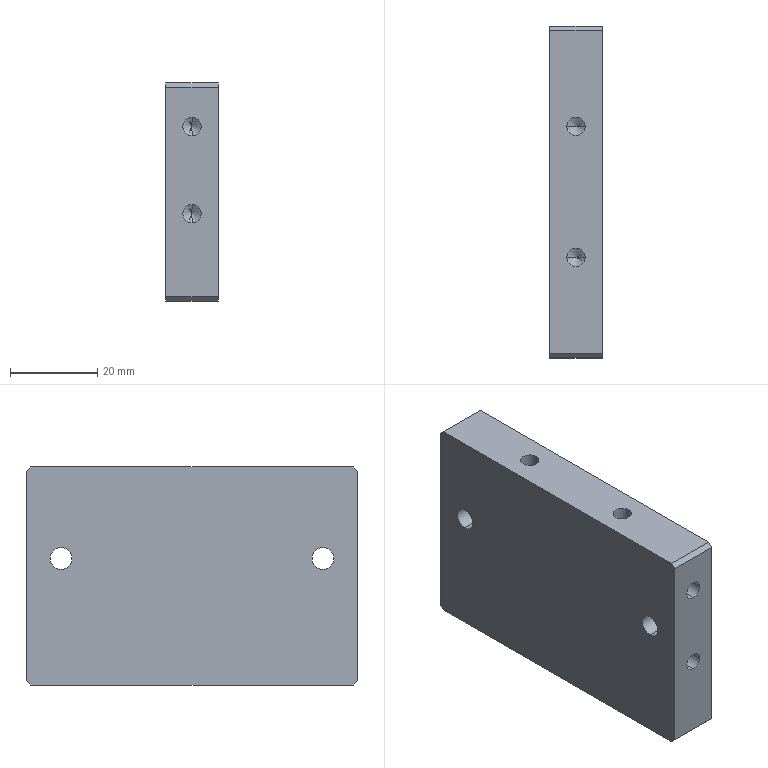Part | SolidWorks | features HoleWzd 3, Chamfer 1, ICE 1, MirrorPattern 1 | 1 solid | 38 faces | box 12 x 76 x 50 mm | volume 43762 mm3 | cylinder 16 | cone 12 | plane 10 | commonest cylinder face diameters 4.2 x12 5 x4
STEP:
#1=CARTESIAN_POINT('',(-8.1,15.,-12.4));
#2=VERTEX_POINT('',#1);
#3=CARTESIAN_POINT('',(-3.9,15.,-12.4));
#4=VERTEX_POINT('',#3);
#5=CARTESIAN_POINT('',(-6.,15.,-12.4));
#6=DIRECTION('',(0.,0.,1.));
#7=DIRECTION('',(1.,0.,0.));
#8=AXIS2_PLACEMENT_3D('',#5,#6,#7);
#9=CIRCLE('',#8,2.1);
#10=EDGE_CURVE('',#2,#4,#9,.T.);
#11=ORIENTED_EDGE('',*,*,#10,.F.);
#12=CARTESIAN_POINT('',(-8.1,15.,0.));
#13=VERTEX_POINT('',#12);
#14=CARTESIAN_POINT('',(-8.1,15.,0.));
#15=DIRECTION('',(0.,0.,1.));
#16=VECTOR('',#15,1000.);
#17=LINE('',#14,#16);
#18=EDGE_CURVE('',#2,#13,#17,.T.);
#19=ORIENTED_EDGE('',*,*,#18,.T.);
#20=CARTESIAN_POINT('',(-3.9,15.,0.));
#21=VERTEX_POINT('',#20);
#22=CARTESIAN_POINT('',(-6.,15.,0.));
#23=DIRECTION('',(0.,0.,1.));
#24=DIRECTION('',(1.,0.,0.));
#25=AXIS2_PLACEMENT_3D('',#22,#23,#24);
#26=CIRCLE('',#25,2.1);
#27=EDGE_CURVE('',#13,#21,#26,.T.);
#28=ORIENTED_EDGE('',*,*,#27,.T.);
#29=CARTESIAN_POINT('',(-3.9,15.,0.));
#30=DIRECTION('',(0.,0.,1.));
#31=VECTOR('',#30,1000.);
#32=LINE('',#29,#31);
#33=EDGE_CURVE('',#4,#21,#32,.T.);
#34=ORIENTED_EDGE('',*,*,#33,.F.);
#35=EDGE_LOOP('',(#11,#19,#28,#34));
#36=FACE_OUTER_BOUND('',#35,.T.);
#37=CARTESIAN_POINT('',(-6.,15.,0.));
#38=DIRECTION('',(0.,0.,1.));
#39=DIRECTION('',(1.,0.,0.));
#40=AXIS2_PLACEMENT_3D('',#37,#38,#39);
#41=CYLINDRICAL_SURFACE('',#40,2.1);
#42=ADVANCED_FACE('',(#36),#41,.F.);
#43=CARTESIAN_POINT('',(-6.,15.,-13.662));
#44=VERTEX_POINT('',#43);
#45=CARTESIAN_POINT('',(-3.9,15.,-12.4));
#46=DIRECTION('',(0.8572,0.,0.515));
#47=VECTOR('',#46,1000.);
#48=LINE('',#45,#47);
#49=EDGE_CURVE('',#44,#4,#48,.T.);
#50=ORIENTED_EDGE('',*,*,#49,.F.);
#51=CARTESIAN_POINT('',(-8.1,15.,-12.4));
#52=DIRECTION('',(-0.8572,0.,0.515));
#53=VECTOR('',#52,1000.);
#54=LINE('',#51,#53);
#55=EDGE_CURVE('',#44,#2,#54,.T.);
#56=ORIENTED_EDGE('',*,*,#55,.T.);
#57=ORIENTED_EDGE('',*,*,#10,.T.);
#58=EDGE_LOOP('',(#50,#56,#57));
#59=FACE_OUTER_BOUND('',#58,.T.);
#60=CARTESIAN_POINT('',(-6.,15.,-12.4));
#61=DIRECTION('',(0.,0.,1.));
#62=DIRECTION('',(1.,0.,0.));
#63=AXIS2_PLACEMENT_3D('',#60,#61,#62);
#64=CONICAL_SURFACE('',#63,2.1,1.03);
#65=ADVANCED_FACE('',(#59),#64,.F.);
#66=CARTESIAN_POINT('',(-8.1,-15.,-12.4));
#67=VERTEX_POINT('',#66);
#68=CARTESIAN_POINT('',(-3.9,-15.,-12.4));
#69=VERTEX_POINT('',#68);
#70=CARTESIAN_POINT('',(-6.,-15.,-12.4));
#71=DIRECTION('',(0.,0.,1.));
#72=DIRECTION('',(1.,0.,0.));
#73=AXIS2_PLACEMENT_3D('',#70,#71,#72);
#74=CIRCLE('',#73,2.1);
#75=EDGE_CURVE('',#67,#69,#74,.T.);
#76=ORIENTED_EDGE('',*,*,#75,.F.);
#77=CARTESIAN_POINT('',(-8.1,-15.,0.));
#78=VERTEX_POINT('',#77);
#79=CARTESIAN_POINT('',(-8.1,-15.,0.));
#80=DIRECTION('',(0.,0.,1.));
#81=VECTOR('',#80,1000.);
#82=LINE('',#79,#81);
#83=EDGE_CURVE('',#67,#78,#82,.T.);
#84=ORIENTED_EDGE('',*,*,#83,.T.);
#85=CARTESIAN_POINT('',(-3.9,-15.,0.));
#86=VERTEX_POINT('',#85);
#87=CARTESIAN_POINT('',(-6.,-15.,0.));
#88=DIRECTION('',(0.,0.,1.));
#89=DIRECTION('',(1.,0.,0.));
#90=AXIS2_PLACEMENT_3D('',#87,#88,#89);
#91=CIRCLE('',#90,2.1);
#92=EDGE_CURVE('',#78,#86,#91,.T.);
#93=ORIENTED_EDGE('',*,*,#92,.T.);
#94=CARTESIAN_POINT('',(-3.9,-15.,0.));
#95=DIRECTION('',(0.,0.,1.));
#96=VECTOR('',#95,1000.);
#97=LINE('',#94,#96);
#98=EDGE_CURVE('',#69,#86,#97,.T.);
#99=ORIENTED_EDGE('',*,*,#98,.F.);
#100=EDGE_LOOP('',(#76,#84,#93,#99));
#101=FACE_OUTER_BOUND('',#100,.T.);
#102=CARTESIAN_POINT('',(-6.,-15.,0.));
#103=DIRECTION('',(0.,0.,1.));
#104=DIRECTION('',(1.,0.,0.));
#105=AXIS2_PLACEMENT_3D('',#102,#103,#104);
#106=CYLINDRICAL_SURFACE('',#105,2.1);
#107=ADVANCED_FACE('',(#101),#106,.F.);
#108=CARTESIAN_POINT('',(-6.,-15.,-13.662));
#109=VERTEX_POINT('',#108);
#110=CARTESIAN_POINT('',(-3.9,-15.,-12.4));
#111=DIRECTION('',(0.8572,0.,0.515));
#112=VECTOR('',#111,1000.);
#113=LINE('',#110,#112);
#114=EDGE_CURVE('',#109,#69,#113,.T.);
#115=ORIENTED_EDGE('',*,*,#114,.F.);
#116=CARTESIAN_POINT('',(-8.1,-15.,-12.4));
#117=DIRECTION('',(-0.8572,0.,0.515));
#118=VECTOR('',#117,1000.);
#119=LINE('',#116,#118);
#120=EDGE_CURVE('',#109,#67,#119,.T.);
#121=ORIENTED_EDGE('',*,*,#120,.T.);
#122=ORIENTED_EDGE('',*,*,#75,.T.);
#123=EDGE_LOOP('',(#115,#121,#122));
#124=FACE_OUTER_BOUND('',#123,.T.);
#125=CARTESIAN_POINT('',(-6.,-15.,-12.4));
#126=DIRECTION('',(0.,0.,1.));
#127=DIRECTION('',(1.,0.,0.));
#128=AXIS2_PLACEMENT_3D('',#125,#126,#127);
#129=CONICAL_SURFACE('',#128,2.1,1.03);
#130=ADVANCED_FACE('',(#124),#129,.F.);
#131=CARTESIAN_POINT('',(-6.,20.6,-12.1));
#132=VERTEX_POINT('',#131);
#133=CARTESIAN_POINT('',(-6.,20.6,-7.9));
#134=VERTEX_POINT('',#133);
#135=CARTESIAN_POINT('',(-6.,20.6,-10.));
#136=DIRECTION('',(0.,1.,0.));
#137=DIRECTION('',(0.,0.,1.));
#138=AXIS2_PLACEMENT_3D('',#135,#136,#137);
#139=CIRCLE('',#138,2.1);
#140=EDGE_CURVE('',#132,#134,#139,.T.);
#141=ORIENTED_EDGE('',*,*,#140,.F.);
#142=CARTESIAN_POINT('',(-6.,38.,-12.1));
#143=VERTEX_POINT('',#142);
#144=CARTESIAN_POINT('',(-6.,38.,-12.1));
#145=DIRECTION('',(0.,1.,0.));
#146=VECTOR('',#145,1000.);
#147=LINE('',#144,#146);
#148=EDGE_CURVE('',#132,#143,#147,.T.);
#149=ORIENTED_EDGE('',*,*,#148,.T.);
#150=CARTESIAN_POINT('',(-6.,38.,-7.9));
#151=VERTEX_POINT('',#150);
#152=CARTESIAN_POINT('',(-6.,38.,-10.));
#153=DIRECTION('',(0.,1.,0.));
#154=DIRECTION('',(0.,0.,1.));
#155=AXIS2_PLACEMENT_3D('',#152,#153,#154);
#156=CIRCLE('',#155,2.1);
#157=EDGE_CURVE('',#143,#151,#156,.T.);
#158=ORIENTED_EDGE('',*,*,#157,.T.);
#159=CARTESIAN_POINT('',(-6.,38.,-7.9));
#160=DIRECTION('',(0.,1.,0.));
#161=VECTOR('',#160,1000.);
#162=LINE('',#159,#161);
#163=EDGE_CURVE('',#134,#151,#162,.T.);
#164=ORIENTED_EDGE('',*,*,#163,.F.);
#165=EDGE_LOOP('',(#141,#149,#158,#164));
#166=FACE_OUTER_BOUND('',#165,.T.);
#167=CARTESIAN_POINT('',(-6.,38.,-10.));
#168=DIRECTION('',(0.,1.,0.));
#169=DIRECTION('',(0.,0.,1.));
#170=AXIS2_PLACEMENT_3D('',#167,#168,#169);
#171=CYLINDRICAL_SURFACE('',#170,2.1);
#172=ADVANCED_FACE('',(#166),#171,.F.);
#173=CARTESIAN_POINT('',(-6.,19.338,-10.));
#174=VERTEX_POINT('',#173);
#175=CARTESIAN_POINT('',(-6.,20.6,-7.9));
#176=DIRECTION('',(0.,0.515,0.8572));
#177=VECTOR('',#176,1000.);
#178=LINE('',#175,#177);
#179=EDGE_CURVE('',#174,#134,#178,.T.);
#180=ORIENTED_EDGE('',*,*,#179,.F.);
#181=CARTESIAN_POINT('',(-6.,20.6,-12.1));
#182=DIRECTION('',(0.,0.515,-0.8572));
#183=VECTOR('',#182,1000.);
#184=LINE('',#181,#183);
#185=EDGE_CURVE('',#174,#132,#184,.T.);
#186=ORIENTED_EDGE('',*,*,#185,.T.);
#187=ORIENTED_EDGE('',*,*,#140,.T.);
#188=EDGE_LOOP('',(#180,#186,#187));
#189=FACE_OUTER_BOUND('',#188,.T.);
#190=CARTESIAN_POINT('',(-6.,20.6,-10.));
#191=DIRECTION('',(0.,1.,0.));
#192=DIRECTION('',(0.,0.,1.));
#193=AXIS2_PLACEMENT_3D('',#190,#191,#192);
#194=CONICAL_SURFACE('',#193,2.1,1.03);
#195=ADVANCED_FACE('',(#189),#194,.F.);
#196=CARTESIAN_POINT('',(-6.,20.6,-32.1));
#197=VERTEX_POINT('',#196);
#198=CARTESIAN_POINT('',(-6.,20.6,-27.9));
#199=VERTEX_POINT('',#198);
#200=CARTESIAN_POINT('',(-6.,20.6,-30.));
#201=DIRECTION('',(0.,1.,0.));
#202=DIRECTION('',(0.,0.,1.));
#203=AXIS2_PLACEMENT_3D('',#200,#201,#202);
#204=CIRCLE('',#203,2.1);
#205=EDGE_CURVE('',#197,#199,#204,.T.);
#206=ORIENTED_EDGE('',*,*,#205,.F.);
#207=CARTESIAN_POINT('',(-6.,38.,-32.1));
#208=VERTEX_POINT('',#207);
#209=CARTESIAN_POINT('',(-6.,38.,-32.1));
#210=DIRECTION('',(0.,1.,0.));
#211=VECTOR('',#210,1000.);
#212=LINE('',#209,#211);
#213=EDGE_CURVE('',#197,#208,#212,.T.);
#214=ORIENTED_EDGE('',*,*,#213,.T.);
#215=CARTESIAN_POINT('',(-6.,38.,-27.9));
#216=VERTEX_POINT('',#215);
#217=CARTESIAN_POINT('',(-6.,38.,-30.));
#218=DIRECTION('',(0.,1.,0.));
#219=DIRECTION('',(0.,0.,1.));
#220=AXIS2_PLACEMENT_3D('',#217,#218,#219);
#221=CIRCLE('',#220,2.1);
#222=EDGE_CURVE('',#208,#216,#221,.T.);
#223=ORIENTED_EDGE('',*,*,#222,.T.);
#224=CARTESIAN_POINT('',(-6.,38.,-27.9));
#225=DIRECTION('',(0.,1.,0.));
#226=VECTOR('',#225,1000.);
#227=LINE('',#224,#226);
#228=EDGE_CURVE('',#199,#216,#227,.T.);
#229=ORIENTED_EDGE('',*,*,#228,.F.);
#230=EDGE_LOOP('',(#206,#214,#223,#229));
#231=FACE_OUTER_BOUND('',#230,.T.);
#232=CARTESIAN_POINT('',(-6.,38.,-30.));
#233=DIRECTION('',(0.,1.,0.));
#234=DIRECTION('',(0.,0.,1.));
#235=AXIS2_PLACEMENT_3D('',#232,#233,#234);
#236=CYLINDRICAL_SURFACE('',#235,2.1);
#237=ADVANCED_FACE('',(#231),#236,.F.);
#238=CARTESIAN_POINT('',(-6.,19.338,-30.));
#239=VERTEX_POINT('',#238);
#240=CARTESIAN_POINT('',(-6.,20.6,-27.9));
#241=DIRECTION('',(0.,0.515,0.8572));
#242=VECTOR('',#241,1000.);
#243=LINE('',#240,#242);
#244=EDGE_CURVE('',#239,#199,#243,.T.);
#245=ORIENTED_EDGE('',*,*,#244,.F.);
#246=CARTESIAN_POINT('',(-6.,20.6,-32.1));
#247=DIRECTION('',(0.,0.515,-0.8572));
#248=VECTOR('',#247,1000.);
#249=LINE('',#246,#248);
#250=EDGE_CURVE('',#239,#197,#249,.T.);
#251=ORIENTED_EDGE('',*,*,#250,.T.);
#252=ORIENTED_EDGE('',*,*,#205,.T.);
#253=EDGE_LOOP('',(#245,#251,#252));
#254=FACE_OUTER_BOUND('',#253,.T.);
#255=CARTESIAN_POINT('',(-6.,20.6,-30.));
#256=DIRECTION('',(0.,1.,0.));
#257=DIRECTION('',(0.,0.,1.));
#258=AXIS2_PLACEMENT_3D('',#255,#256,#257);
#259=CONICAL_SURFACE('',#258,2.1,1.03);
#260=ADVANCED_FACE('',(#254),#259,.F.);
#261=CARTESIAN_POINT('',(-6.,-20.6,-7.9));
#262=VERTEX_POINT('',#261);
#263=CARTESIAN_POINT('',(-6.,-20.6,-12.1));
#264=VERTEX_POINT('',#263);
#265=CARTESIAN_POINT('',(-6.,-20.6,-10.));
#266=DIRECTION('',(0.,-1.,0.));
#267=DIRECTION('',(0.,0.,-1.));
#268=AXIS2_PLACEMENT_3D('',#265,#266,#267);
#269=CIRCLE('',#268,2.1);
#270=EDGE_CURVE('',#262,#264,#269,.T.);
#271=ORIENTED_EDGE('',*,*,#270,.F.);
#272=CARTESIAN_POINT('',(-6.,-38.,-7.9));
#273=VERTEX_POINT('',#272);
#274=CARTESIAN_POINT('',(-6.,-38.,-7.9));
#275=DIRECTION('',(0.,-1.,0.));
#276=VECTOR('',#275,1000.);
#277=LINE('',#274,#276);
#278=EDGE_CURVE('',#262,#273,#277,.T.);
#279=ORIENTED_EDGE('',*,*,#278,.T.);
#280=CARTESIAN_POINT('',(-6.,-38.,-12.1));
#281=VERTEX_POINT('',#280);
#282=CARTESIAN_POINT('',(-6.,-38.,-10.));
#283=DIRECTION('',(0.,-1.,0.));
#284=DIRECTION('',(0.,0.,-1.));
#285=AXIS2_PLACEMENT_3D('',#282,#283,#284);
#286=CIRCLE('',#285,2.1);
#287=EDGE_CURVE('',#273,#281,#286,.T.);
#288=ORIENTED_EDGE('',*,*,#287,.T.);
#289=CARTESIAN_POINT('',(-6.,-38.,-12.1));
#290=DIRECTION('',(0.,-1.,0.));
#291=VECTOR('',#290,1000.);
#292=LINE('',#289,#291);
#293=EDGE_CURVE('',#264,#281,#292,.T.);
#294=ORIENTED_EDGE('',*,*,#293,.F.);
#295=EDGE_LOOP('',(#271,#279,#288,#294));
#296=FACE_OUTER_BOUND('',#295,.T.);
#297=CARTESIAN_POINT('',(-6.,-38.,-10.));
#298=DIRECTION('',(0.,-1.,0.));
#299=DIRECTION('',(0.,0.,-1.));
#300=AXIS2_PLACEMENT_3D('',#297,#298,#299);
#301=CYLINDRICAL_SURFACE('',#300,2.1);
#302=ADVANCED_FACE('',(#296),#301,.F.);
#303=CARTESIAN_POINT('',(-6.,-19.338,-10.));
#304=VERTEX_POINT('',#303);
#305=CARTESIAN_POINT('',(-6.,-20.6,-12.1));
#306=DIRECTION('',(0.,-0.515,-0.8572));
#307=VECTOR('',#306,1000.);
#308=LINE('',#305,#307);
#309=EDGE_CURVE('',#304,#264,#308,.T.);
#310=ORIENTED_EDGE('',*,*,#309,.F.);
#311=CARTESIAN_POINT('',(-6.,-20.6,-7.9));
#312=DIRECTION('',(0.,-0.515,0.8572));
#313=VECTOR('',#312,1000.);
#314=LINE('',#311,#313);
#315=EDGE_CURVE('',#304,#262,#314,.T.);
#316=ORIENTED_EDGE('',*,*,#315,.T.);
#317=ORIENTED_EDGE('',*,*,#270,.T.);
#318=EDGE_LOOP('',(#310,#316,#317));
#319=FACE_OUTER_BOUND('',#318,.T.);
#320=CARTESIAN_POINT('',(-6.,-20.6,-10.));
#321=DIRECTION('',(0.,-1.,0.));
#322=DIRECTION('',(0.,0.,-1.));
#323=AXIS2_PLACEMENT_3D('',#320,#321,#322);
#324=CONICAL_SURFACE('',#323,2.1,1.03);
#325=ADVANCED_FACE('',(#319),#324,.F.);
#326=CARTESIAN_POINT('',(-6.,-20.6,-27.9));
#327=VERTEX_POINT('',#326);
#328=CARTESIAN_POINT('',(-6.,-20.6,-32.1));
#329=VERTEX_POINT('',#328);
#330=CARTESIAN_POINT('',(-6.,-20.6,-30.));
#331=DIRECTION('',(0.,-1.,0.));
#332=DIRECTION('',(0.,0.,-1.));
#333=AXIS2_PLACEMENT_3D('',#330,#331,#332);
#334=CIRCLE('',#333,2.1);
#335=EDGE_CURVE('',#327,#329,#334,.T.);
#336=ORIENTED_EDGE('',*,*,#335,.F.);
#337=CARTESIAN_POINT('',(-6.,-38.,-27.9));
#338=VERTEX_POINT('',#337);
#339=CARTESIAN_POINT('',(-6.,-38.,-27.9));
#340=DIRECTION('',(0.,-1.,0.));
#341=VECTOR('',#340,1000.);
#342=LINE('',#339,#341);
#343=EDGE_CURVE('',#327,#338,#342,.T.);
#344=ORIENTED_EDGE('',*,*,#343,.T.);
#345=CARTESIAN_POINT('',(-6.,-38.,-32.1));
#346=VERTEX_POINT('',#345);
#347=CARTESIAN_POINT('',(-6.,-38.,-30.));
#348=DIRECTION('',(0.,-1.,0.));
#349=DIRECTION('',(0.,0.,-1.));
#350=AXIS2_PLACEMENT_3D('',#347,#348,#349);
#351=CIRCLE('',#350,2.1);
#352=EDGE_CURVE('',#338,#346,#351,.T.);
#353=ORIENTED_EDGE('',*,*,#352,.T.);
#354=CARTESIAN_POINT('',(-6.,-38.,-32.1));
#355=DIRECTION('',(0.,-1.,0.));
#356=VECTOR('',#355,1000.);
#357=LINE('',#354,#356);
#358=EDGE_CURVE('',#329,#346,#357,.T.);
#359=ORIENTED_EDGE('',*,*,#358,.F.);
#360=EDGE_LOOP('',(#336,#344,#353,#359));
#361=FACE_OUTER_BOUND('',#360,.T.);
#362=CARTESIAN_POINT('',(-6.,-38.,-30.));
#363=DIRECTION('',(0.,-1.,0.));
#364=DIRECTION('',(0.,0.,-1.));
#365=AXIS2_PLACEMENT_3D('',#362,#363,#364);
#366=CYLINDRICAL_SURFACE('',#365,2.1);
#367=ADVANCED_FACE('',(#361),#366,.F.);
#368=CARTESIAN_POINT('',(-6.,-19.338,-30.));
#369=VERTEX_POINT('',#368);
#370=CARTESIAN_POINT('',(-6.,-20.6,-32.1));
#371=DIRECTION('',(0.,-0.515,-0.8572));
#372=VECTOR('',#371,1000.);
#373=LINE('',#370,#372);
#374=EDGE_CURVE('',#369,#329,#373,.T.);
#375=ORIENTED_EDGE('',*,*,#374,.F.);
#376=CARTESIAN_POINT('',(-6.,-20.6,-27.9));
#377=DIRECTION('',(0.,-0.515,0.8572));
#378=VECTOR('',#377,1000.);
#379=LINE('',#376,#378);
#380=EDGE_CURVE('',#369,#327,#379,.T.);
#381=ORIENTED_EDGE('',*,*,#380,.T.);
#382=ORIENTED_EDGE('',*,*,#335,.T.);
#383=EDGE_LOOP('',(#375,#381,#382));
#384=FACE_OUTER_BOUND('',#383,.T.);
#385=CARTESIAN_POINT('',(-6.,-20.6,-30.));
#386=DIRECTION('',(0.,-1.,0.));
#387=DIRECTION('',(0.,0.,-1.));
#388=AXIS2_PLACEMENT_3D('',#385,#386,#387);
#389=CONICAL_SURFACE('',#388,2.1,1.03);
#390=ADVANCED_FACE('',(#384),#389,.F.);
#391=CARTESIAN_POINT('',(-12.,-30.,-18.5));
#392=VERTEX_POINT('',#391);
#393=CARTESIAN_POINT('',(-12.,-30.,-23.5));
#394=VERTEX_POINT('',#393);
#395=CARTESIAN_POINT('',(-12.,-30.,-21.));
#396=DIRECTION('',(1.,0.,0.));
#397=DIRECTION('',(0.,0.,-1.));
#398=AXIS2_PLACEMENT_3D('',#395,#396,#397);
#399=CIRCLE('',#398,2.5);
#400=EDGE_CURVE('',#392,#394,#399,.T.);
#401=ORIENTED_EDGE('',*,*,#400,.F.);
#402=CARTESIAN_POINT('',(0.,-30.,-18.5));
#403=VERTEX_POINT('',#402);
#404=CARTESIAN_POINT('',(0.,-30.,-18.5));
#405=DIRECTION('',(1.,0.,0.));
#406=VECTOR('',#405,1000.);
#407=LINE('',#404,#406);
#408=EDGE_CURVE('',#392,#403,#407,.T.);
#409=ORIENTED_EDGE('',*,*,#408,.T.);
#410=CARTESIAN_POINT('',(0.,-30.,-23.5));
#411=VERTEX_POINT('',#410);
#412=CARTESIAN_POINT('',(0.,-30.,-21.));
#413=DIRECTION('',(1.,0.,0.));
#414=DIRECTION('',(0.,0.,-1.));
#415=AXIS2_PLACEMENT_3D('',#412,#413,#414);
#416=CIRCLE('',#415,2.5);
#417=EDGE_CURVE('',#403,#411,#416,.T.);
#418=ORIENTED_EDGE('',*,*,#417,.T.);
#419=CARTESIAN_POINT('',(0.,-30.,-23.5));
#420=DIRECTION('',(1.,0.,0.));
#421=VECTOR('',#420,1000.);
#422=LINE('',#419,#421);
#423=EDGE_CURVE('',#394,#411,#422,.T.);
#424=ORIENTED_EDGE('',*,*,#423,.F.);
#425=EDGE_LOOP('',(#401,#409,#418,#424));
#426=FACE_OUTER_BOUND('',#425,.T.);
#427=CARTESIAN_POINT('',(0.,-30.,-21.));
#428=DIRECTION('',(1.,0.,0.));
#429=DIRECTION('',(0.,0.,-1.));
#430=AXIS2_PLACEMENT_3D('',#427,#428,#429);
#431=CYLINDRICAL_SURFACE('',#430,2.5);
#432=ADVANCED_FACE('',(#426),#431,.F.);
#433=CARTESIAN_POINT('',(-12.,30.,-18.5));
#434=VERTEX_POINT('',#433);
#435=CARTESIAN_POINT('',(-12.,30.,-23.5));
#436=VERTEX_POINT('',#435);
#437=CARTESIAN_POINT('',(-12.,30.,-21.));
#438=DIRECTION('',(1.,0.,0.));
#439=DIRECTION('',(0.,0.,-1.));
#440=AXIS2_PLACEMENT_3D('',#437,#438,#439);
#441=CIRCLE('',#440,2.5);
#442=EDGE_CURVE('',#434,#436,#441,.T.);
#443=ORIENTED_EDGE('',*,*,#442,.F.);
#444=CARTESIAN_POINT('',(0.,30.,-18.5));
#445=VERTEX_POINT('',#444);
#446=CARTESIAN_POINT('',(0.,30.,-18.5));
#447=DIRECTION('',(1.,0.,0.));
#448=VECTOR('',#447,1000.);
#449=LINE('',#446,#448);
#450=EDGE_CURVE('',#434,#445,#449,.T.);
#451=ORIENTED_EDGE('',*,*,#450,.T.);
#452=CARTESIAN_POINT('',(0.,30.,-23.5));
#453=VERTEX_POINT('',#452);
#454=CARTESIAN_POINT('',(0.,30.,-21.));
#455=DIRECTION('',(1.,0.,0.));
#456=DIRECTION('',(0.,0.,-1.));
#457=AXIS2_PLACEMENT_3D('',#454,#455,#456);
#458=CIRCLE('',#457,2.5);
#459=EDGE_CURVE('',#445,#453,#458,.T.);
#460=ORIENTED_EDGE('',*,*,#459,.T.);
#461=CARTESIAN_POINT('',(0.,30.,-23.5));
#462=DIRECTION('',(1.,0.,0.));
#463=VECTOR('',#462,1000.);
#464=LINE('',#461,#463);
#465=EDGE_CURVE('',#436,#453,#464,.T.);
#466=ORIENTED_EDGE('',*,*,#465,.F.);
#467=EDGE_LOOP('',(#443,#451,#460,#466));
#468=FACE_OUTER_BOUND('',#467,.T.);
#469=CARTESIAN_POINT('',(0.,30.,-21.));
#470=DIRECTION('',(1.,0.,0.));
#471=DIRECTION('',(0.,0.,-1.));
#472=AXIS2_PLACEMENT_3D('',#469,#470,#471);
#473=CYLINDRICAL_SURFACE('',#472,2.5);
#474=ADVANCED_FACE('',(#468),#473,.F.);
#475=CARTESIAN_POINT('',(-6.,15.,0.));
#476=DIRECTION('',(0.,0.,1.));
#477=DIRECTION('',(1.,0.,0.));
#478=AXIS2_PLACEMENT_3D('',#475,#476,#477);
#479=CIRCLE('',#478,2.1);
#480=EDGE_CURVE('',#21,#13,#479,.T.);
#481=ORIENTED_EDGE('',*,*,#480,.F.);
#482=ORIENTED_EDGE('',*,*,#27,.F.);
#483=EDGE_LOOP('',(#481,#482));
#484=FACE_BOUND('',#483,.T.);
#485=CARTESIAN_POINT('',(-6.,-15.,0.));
#486=DIRECTION('',(0.,0.,1.));
#487=DIRECTION('',(1.,0.,0.));
#488=AXIS2_PLACEMENT_3D('',#485,#486,#487);
#489=CIRCLE('',#488,2.1);
#490=EDGE_CURVE('',#86,#78,#489,.T.);
#491=ORIENTED_EDGE('',*,*,#490,.F.);
#492=ORIENTED_EDGE('',*,*,#92,.F.);
#493=EDGE_LOOP('',(#491,#492));
#494=FACE_BOUND('',#493,.T.);
#495=CARTESIAN_POINT('',(0.,37.,0.));
#496=VERTEX_POINT('',#495);
#497=CARTESIAN_POINT('',(0.,-37.,0.));
#498=VERTEX_POINT('',#497);
#499=CARTESIAN_POINT('',(0.,38.,0.));
#500=DIRECTION('',(0.,-1.,0.));
#501=VECTOR('',#500,1000.);
#502=LINE('',#499,#501);
#503=EDGE_CURVE('',#496,#498,#502,.T.);
#504=ORIENTED_EDGE('',*,*,#503,.F.);
#505=CARTESIAN_POINT('',(-12.,37.,0.));
#506=VERTEX_POINT('',#505);
#507=CARTESIAN_POINT('',(-12.,37.,0.));
#508=DIRECTION('',(-1.,0.,0.));
#509=VECTOR('',#508,1000.);
#510=LINE('',#507,#509);
#511=EDGE_CURVE('',#496,#506,#510,.T.);
#512=ORIENTED_EDGE('',*,*,#511,.T.);
#513=CARTESIAN_POINT('',(-12.,-37.,0.));
#514=VERTEX_POINT('',#513);
#515=CARTESIAN_POINT('',(-12.,38.,0.));
#516=DIRECTION('',(0.,-1.,0.));
#517=VECTOR('',#516,1000.);
#518=LINE('',#515,#517);
#519=EDGE_CURVE('',#506,#514,#518,.T.);
#520=ORIENTED_EDGE('',*,*,#519,.T.);
#521=CARTESIAN_POINT('',(-12.,-37.,0.));
#522=DIRECTION('',(1.,0.,0.));
#523=VECTOR('',#522,1000.);
#524=LINE('',#521,#523);
#525=EDGE_CURVE('',#514,#498,#524,.T.);
#526=ORIENTED_EDGE('',*,*,#525,.T.);
#527=EDGE_LOOP('',(#504,#512,#520,#526));
#528=FACE_OUTER_BOUND('',#527,.T.);
#529=CARTESIAN_POINT('',(-12.,38.,0.));
#530=DIRECTION('',(0.,0.,1.));
#531=DIRECTION('',(1.,0.,0.));
#532=AXIS2_PLACEMENT_3D('',#529,#530,#531);
#533=PLANE('',#532);
#534=ADVANCED_FACE('',(#484,#494,#528),#533,.T.);
#535=CARTESIAN_POINT('',(-6.,38.,-10.));
#536=DIRECTION('',(0.,1.,0.));
#537=DIRECTION('',(0.,0.,1.));
#538=AXIS2_PLACEMENT_3D('',#535,#536,#537);
#539=CIRCLE('',#538,2.1);
#540=EDGE_CURVE('',#151,#143,#539,.T.);
#541=ORIENTED_EDGE('',*,*,#540,.F.);
#542=ORIENTED_EDGE('',*,*,#157,.F.);
#543=EDGE_LOOP('',(#541,#542));
#544=FACE_BOUND('',#543,.T.);
#545=CARTESIAN_POINT('',(-6.,38.,-30.));
#546=DIRECTION('',(0.,1.,0.));
#547=DIRECTION('',(0.,0.,1.));
#548=AXIS2_PLACEMENT_3D('',#545,#546,#547);
#549=CIRCLE('',#548,2.1);
#550=EDGE_CURVE('',#216,#208,#549,.T.);
#551=ORIENTED_EDGE('',*,*,#550,.F.);
#552=ORIENTED_EDGE('',*,*,#222,.F.);
#553=EDGE_LOOP('',(#551,#552));
#554=FACE_BOUND('',#553,.T.);
#555=CARTESIAN_POINT('',(-12.,38.,-49.));
#556=VERTEX_POINT('',#555);
#557=CARTESIAN_POINT('',(-12.,38.,-1.));
#558=VERTEX_POINT('',#557);
#559=CARTESIAN_POINT('',(-12.,38.,0.));
#560=DIRECTION('',(0.,0.,1.));
#561=VECTOR('',#560,1000.);
#562=LINE('',#559,#561);
#563=EDGE_CURVE('',#556,#558,#562,.T.);
#564=ORIENTED_EDGE('',*,*,#563,.T.);
#565=CARTESIAN_POINT('',(0.,38.,-1.));
#566=VERTEX_POINT('',#565);
#567=CARTESIAN_POINT('',(-12.,38.,-1.));
#568=DIRECTION('',(1.,0.,0.));
#569=VECTOR('',#568,1000.);
#570=LINE('',#567,#569);
#571=EDGE_CURVE('',#558,#566,#570,.T.);
#572=ORIENTED_EDGE('',*,*,#571,.T.);
#573=CARTESIAN_POINT('',(0.,38.,-49.));
#574=VERTEX_POINT('',#573);
#575=CARTESIAN_POINT('',(0.,38.,0.));
#576=DIRECTION('',(0.,0.,1.));
#577=VECTOR('',#576,1000.);
#578=LINE('',#575,#577);
#579=EDGE_CURVE('',#574,#566,#578,.T.);
#580=ORIENTED_EDGE('',*,*,#579,.F.);
#581=CARTESIAN_POINT('',(-12.,38.,-49.));
#582=DIRECTION('',(-1.,0.,0.));
#583=VECTOR('',#582,1000.);
#584=LINE('',#581,#583);
#585=EDGE_CURVE('',#574,#556,#584,.T.);
#586=ORIENTED_EDGE('',*,*,#585,.T.);
#587=EDGE_LOOP('',(#564,#572,#580,#586));
#588=FACE_OUTER_BOUND('',#587,.T.);
#589=CARTESIAN_POINT('',(-12.,38.,0.));
#590=DIRECTION('',(0.,1.,0.));
#591=DIRECTION('',(0.,0.,1.));
#592=AXIS2_PLACEMENT_3D('',#589,#590,#591);
#593=PLANE('',#592);
#594=ADVANCED_FACE('',(#544,#554,#588),#593,.T.);
#595=CARTESIAN_POINT('',(-12.,-37.,-50.));
#596=VERTEX_POINT('',#595);
#597=CARTESIAN_POINT('',(-12.,37.,-50.));
#598=VERTEX_POINT('',#597);
#599=CARTESIAN_POINT('',(-12.,38.,-50.));
#600=DIRECTION('',(0.,1.,0.));
#601=VECTOR('',#600,1000.);
#602=LINE('',#599,#601);
#603=EDGE_CURVE('',#596,#598,#602,.T.);
#604=ORIENTED_EDGE('',*,*,#603,.T.);
#605=CARTESIAN_POINT('',(0.,37.,-50.));
#606=VERTEX_POINT('',#605);
#607=CARTESIAN_POINT('',(-12.,37.,-50.));
#608=DIRECTION('',(1.,0.,0.));
#609=VECTOR('',#608,1000.);
#610=LINE('',#607,#609);
#611=EDGE_CURVE('',#598,#606,#610,.T.);
#612=ORIENTED_EDGE('',*,*,#611,.T.);
#613=CARTESIAN_POINT('',(0.,-37.,-50.));
#614=VERTEX_POINT('',#613);
#615=CARTESIAN_POINT('',(0.,38.,-50.));
#616=DIRECTION('',(0.,1.,0.));
#617=VECTOR('',#616,1000.);
#618=LINE('',#615,#617);
#619=EDGE_CURVE('',#614,#606,#618,.T.);
#620=ORIENTED_EDGE('',*,*,#619,.F.);
#621=CARTESIAN_POINT('',(-12.,-37.,-50.));
#622=DIRECTION('',(-1.,0.,0.));
#623=VECTOR('',#622,1000.);
#624=LINE('',#621,#623);
#625=EDGE_CURVE('',#614,#596,#624,.T.);
#626=ORIENTED_EDGE('',*,*,#625,.T.);
#627=EDGE_LOOP('',(#604,#612,#620,#626));
#628=FACE_OUTER_BOUND('',#627,.T.);
#629=CARTESIAN_POINT('',(-12.,38.,-50.));
#630=DIRECTION('',(0.,0.,-1.));
#631=DIRECTION('',(-1.,0.,0.));
#632=AXIS2_PLACEMENT_3D('',#629,#630,#631);
#633=PLANE('',#632);
#634=ADVANCED_FACE('',(#628),#633,.T.);
#635=CARTESIAN_POINT('',(-6.,-38.,-10.));
#636=DIRECTION('',(0.,-1.,0.));
#637=DIRECTION('',(0.,0.,-1.));
#638=AXIS2_PLACEMENT_3D('',#635,#636,#637);
#639=CIRCLE('',#638,2.1);
#640=EDGE_CURVE('',#281,#273,#639,.T.);
#641=ORIENTED_EDGE('',*,*,#640,.F.);
#642=ORIENTED_EDGE('',*,*,#287,.F.);
#643=EDGE_LOOP('',(#641,#642));
#644=FACE_BOUND('',#643,.T.);
#645=CARTESIAN_POINT('',(-6.,-38.,-30.));
#646=DIRECTION('',(0.,-1.,0.));
#647=DIRECTION('',(0.,0.,-1.));
#648=AXIS2_PLACEMENT_3D('',#645,#646,#647);
#649=CIRCLE('',#648,2.1);
#650=EDGE_CURVE('',#346,#338,#649,.T.);
#651=ORIENTED_EDGE('',*,*,#650,.F.);
#652=ORIENTED_EDGE('',*,*,#352,.F.);
#653=EDGE_LOOP('',(#651,#652));
#654=FACE_BOUND('',#653,.T.);
#655=CARTESIAN_POINT('',(-12.,-38.,-1.));
#656=VERTEX_POINT('',#655);
#657=CARTESIAN_POINT('',(-12.,-38.,-49.));
#658=VERTEX_POINT('',#657);
#659=CARTESIAN_POINT('',(-12.,-38.,0.));
#660=DIRECTION('',(0.,0.,-1.));
#661=VECTOR('',#660,1000.);
#662=LINE('',#659,#661);
#663=EDGE_CURVE('',#656,#658,#662,.T.);
#664=ORIENTED_EDGE('',*,*,#663,.T.);
#665=CARTESIAN_POINT('',(0.,-38.,-49.));
#666=VERTEX_POINT('',#665);
#667=CARTESIAN_POINT('',(-12.,-38.,-49.));
#668=DIRECTION('',(1.,0.,0.));
#669=VECTOR('',#668,1000.);
#670=LINE('',#667,#669);
#671=EDGE_CURVE('',#658,#666,#670,.T.);
#672=ORIENTED_EDGE('',*,*,#671,.T.);
#673=CARTESIAN_POINT('',(0.,-38.,-1.));
#674=VERTEX_POINT('',#673);
#675=CARTESIAN_POINT('',(0.,-38.,0.));
#676=DIRECTION('',(0.,0.,-1.));
#677=VECTOR('',#676,1000.);
#678=LINE('',#675,#677);
#679=EDGE_CURVE('',#674,#666,#678,.T.);
#680=ORIENTED_EDGE('',*,*,#679,.F.);
#681=CARTESIAN_POINT('',(-12.,-38.,-1.));
#682=DIRECTION('',(-1.,0.,0.));
#683=VECTOR('',#682,1000.);
#684=LINE('',#681,#683);
#685=EDGE_CURVE('',#674,#656,#684,.T.);
#686=ORIENTED_EDGE('',*,*,#685,.T.);
#687=EDGE_LOOP('',(#664,#672,#680,#686));
#688=FACE_OUTER_BOUND('',#687,.T.);
#689=CARTESIAN_POINT('',(-12.,-38.,0.));
#690=DIRECTION('',(0.,-1.,0.));
#691=DIRECTION('',(0.,0.,-1.));
#692=AXIS2_PLACEMENT_3D('',#689,#690,#691);
#693=PLANE('',#692);
#694=ADVANCED_FACE('',(#644,#654,#688),#693,.T.);
#695=CARTESIAN_POINT('',(-12.,-30.,-21.));
#696=DIRECTION('',(1.,0.,0.));
#697=DIRECTION('',(0.,0.,-1.));
#698=AXIS2_PLACEMENT_3D('',#695,#696,#697);
#699=CIRCLE('',#698,2.5);
#700=EDGE_CURVE('',#394,#392,#699,.T.);
#701=ORIENTED_EDGE('',*,*,#700,.T.);
#702=ORIENTED_EDGE('',*,*,#400,.T.);
#703=EDGE_LOOP('',(#701,#702));
#704=FACE_BOUND('',#703,.T.);
#705=CARTESIAN_POINT('',(-12.,30.,-21.));
#706=DIRECTION('',(1.,0.,0.));
#707=DIRECTION('',(0.,0.,-1.));
#708=AXIS2_PLACEMENT_3D('',#705,#706,#707);
#709=CIRCLE('',#708,2.5);
#710=EDGE_CURVE('',#436,#434,#709,.T.);
#711=ORIENTED_EDGE('',*,*,#710,.T.);
#712=ORIENTED_EDGE('',*,*,#442,.T.);
#713=EDGE_LOOP('',(#711,#712));
#714=FACE_BOUND('',#713,.T.);
#715=ORIENTED_EDGE('',*,*,#519,.F.);
#716=CARTESIAN_POINT('',(-12.,38.,-1.));
#717=DIRECTION('',(0.,0.7071,-0.7071));
#718=VECTOR('',#717,1000.);
#719=LINE('',#716,#718);
#720=EDGE_CURVE('',#506,#558,#719,.T.);
#721=ORIENTED_EDGE('',*,*,#720,.T.);
#722=ORIENTED_EDGE('',*,*,#563,.F.);
#723=CARTESIAN_POINT('',(-12.,37.,-50.));
#724=DIRECTION('',(0.,-0.7071,-0.7071));
#725=VECTOR('',#724,1000.);
#726=LINE('',#723,#725);
#727=EDGE_CURVE('',#556,#598,#726,.T.);
#728=ORIENTED_EDGE('',*,*,#727,.T.);
#729=ORIENTED_EDGE('',*,*,#603,.F.);
#730=CARTESIAN_POINT('',(-12.,-38.,-49.));
#731=DIRECTION('',(0.,-0.7071,0.7071));
#732=VECTOR('',#731,1000.);
#733=LINE('',#730,#732);
#734=EDGE_CURVE('',#596,#658,#733,.T.);
#735=ORIENTED_EDGE('',*,*,#734,.T.);
#736=ORIENTED_EDGE('',*,*,#663,.F.);
#737=CARTESIAN_POINT('',(-12.,-37.,0.));
#738=DIRECTION('',(0.,0.7071,0.7071));
#739=VECTOR('',#738,1000.);
#740=LINE('',#737,#739);
#741=EDGE_CURVE('',#656,#514,#740,.T.);
#742=ORIENTED_EDGE('',*,*,#741,.T.);
#743=EDGE_LOOP('',(#715,#721,#722,#728,#729,#735,#736,#742));
#744=FACE_OUTER_BOUND('',#743,.T.);
#745=CARTESIAN_POINT('',(-12.,0.,0.));
#746=DIRECTION('',(1.,0.,0.));
#747=DIRECTION('',(0.,0.,-1.));
#748=AXIS2_PLACEMENT_3D('',#745,#746,#747);
#749=PLANE('',#748);
#750=ADVANCED_FACE('',(#704,#714,#744),#749,.F.);
#751=CARTESIAN_POINT('',(0.,-30.,-21.));
#752=DIRECTION('',(1.,0.,0.));
#753=DIRECTION('',(0.,0.,-1.));
#754=AXIS2_PLACEMENT_3D('',#751,#752,#753);
#755=CIRCLE('',#754,2.5);
#756=EDGE_CURVE('',#411,#403,#755,.T.);
#757=ORIENTED_EDGE('',*,*,#756,.F.);
#758=ORIENTED_EDGE('',*,*,#417,.F.);
#759=EDGE_LOOP('',(#757,#758));
#760=FACE_BOUND('',#759,.T.);
#761=CARTESIAN_POINT('',(0.,30.,-21.));
#762=DIRECTION('',(1.,0.,0.));
#763=DIRECTION('',(0.,0.,-1.));
#764=AXIS2_PLACEMENT_3D('',#761,#762,#763);
#765=CIRCLE('',#764,2.5);
#766=EDGE_CURVE('',#453,#445,#765,.T.);
#767=ORIENTED_EDGE('',*,*,#766,.F.);
#768=ORIENTED_EDGE('',*,*,#459,.F.);
#769=EDGE_LOOP('',(#767,#768));
#770=FACE_BOUND('',#769,.T.);
#771=ORIENTED_EDGE('',*,*,#579,.T.);
#772=CARTESIAN_POINT('',(0.,18.5,18.5));
#773=DIRECTION('',(0.,-0.7071,0.7071));
#774=VECTOR('',#773,1000.);
#775=LINE('',#772,#774);
#776=EDGE_CURVE('',#566,#496,#775,.T.);
#777=ORIENTED_EDGE('',*,*,#776,.T.);
#778=ORIENTED_EDGE('',*,*,#503,.T.);
#779=CARTESIAN_POINT('',(0.,-18.5,18.5));
#780=DIRECTION('',(0.,-0.7071,-0.7071));
#781=VECTOR('',#780,1000.);
#782=LINE('',#779,#781);
#783=EDGE_CURVE('',#498,#674,#782,.T.);
#784=ORIENTED_EDGE('',*,*,#783,.T.);
#785=ORIENTED_EDGE('',*,*,#679,.T.);
#786=CARTESIAN_POINT('',(0.,-43.5,-43.5));
#787=DIRECTION('',(0.,0.7071,-0.7071));
#788=VECTOR('',#787,1000.);
#789=LINE('',#786,#788);
#790=EDGE_CURVE('',#666,#614,#789,.T.);
#791=ORIENTED_EDGE('',*,*,#790,.T.);
#792=ORIENTED_EDGE('',*,*,#619,.T.);
#793=CARTESIAN_POINT('',(0.,43.5,-43.5));
#794=DIRECTION('',(0.,0.7071,0.7071));
#795=VECTOR('',#794,1000.);
#796=LINE('',#793,#795);
#797=EDGE_CURVE('',#606,#574,#796,.T.);
#798=ORIENTED_EDGE('',*,*,#797,.T.);
#799=EDGE_LOOP('',(#771,#777,#778,#784,#785,#791,#792,#798));
#800=FACE_OUTER_BOUND('',#799,.T.);
#801=CARTESIAN_POINT('',(0.,0.,0.));
#802=DIRECTION('',(1.,0.,0.));
#803=DIRECTION('',(0.,0.,-1.));
#804=AXIS2_PLACEMENT_3D('',#801,#802,#803);
#805=PLANE('',#804);
#806=ADVANCED_FACE('',(#760,#770,#800),#805,.T.);
#807=ORIENTED_EDGE('',*,*,#450,.F.);
#808=ORIENTED_EDGE('',*,*,#710,.F.);
#809=ORIENTED_EDGE('',*,*,#465,.T.);
#810=ORIENTED_EDGE('',*,*,#766,.T.);
#811=EDGE_LOOP('',(#807,#808,#809,#810));
#812=FACE_OUTER_BOUND('',#811,.T.);
#813=CARTESIAN_POINT('',(0.,30.,-21.));
#814=DIRECTION('',(1.,0.,0.));
#815=DIRECTION('',(0.,0.,-1.));
#816=AXIS2_PLACEMENT_3D('',#813,#814,#815);
#817=CYLINDRICAL_SURFACE('',#816,2.5);
#818=ADVANCED_FACE('',(#812),#817,.F.);
#819=ORIENTED_EDGE('',*,*,#408,.F.);
#820=ORIENTED_EDGE('',*,*,#700,.F.);
#821=ORIENTED_EDGE('',*,*,#423,.T.);
#822=ORIENTED_EDGE('',*,*,#756,.T.);
#823=EDGE_LOOP('',(#819,#820,#821,#822));
#824=FACE_OUTER_BOUND('',#823,.T.);
#825=CARTESIAN_POINT('',(0.,-30.,-21.));
#826=DIRECTION('',(1.,0.,0.));
#827=DIRECTION('',(0.,0.,-1.));
#828=AXIS2_PLACEMENT_3D('',#825,#826,#827);
#829=CYLINDRICAL_SURFACE('',#828,2.5);
#830=ADVANCED_FACE('',(#824),#829,.F.);
#831=ORIENTED_EDGE('',*,*,#380,.F.);
#832=ORIENTED_EDGE('',*,*,#374,.T.);
#833=CARTESIAN_POINT('',(-6.,-20.6,-30.));
#834=DIRECTION('',(0.,-1.,0.));
#835=DIRECTION('',(0.,0.,-1.));
#836=AXIS2_PLACEMENT_3D('',#833,#834,#835);
#837=CIRCLE('',#836,2.1);
#838=EDGE_CURVE('',#329,#327,#837,.T.);
#839=ORIENTED_EDGE('',*,*,#838,.T.);
#840=EDGE_LOOP('',(#831,#832,#839));
#841=FACE_OUTER_BOUND('',#840,.T.);
#842=CARTESIAN_POINT('',(-6.,-20.6,-30.));
#843=DIRECTION('',(0.,-1.,0.));
#844=DIRECTION('',(0.,0.,-1.));
#845=AXIS2_PLACEMENT_3D('',#842,#843,#844);
#846=CONICAL_SURFACE('',#845,2.1,1.03);
#847=ADVANCED_FACE('',(#841),#846,.F.);
#848=ORIENTED_EDGE('',*,*,#343,.F.);
#849=ORIENTED_EDGE('',*,*,#838,.F.);
#850=ORIENTED_EDGE('',*,*,#358,.T.);
#851=ORIENTED_EDGE('',*,*,#650,.T.);
#852=EDGE_LOOP('',(#848,#849,#850,#851));
#853=FACE_OUTER_BOUND('',#852,.T.);
#854=CARTESIAN_POINT('',(-6.,-38.,-30.));
#855=DIRECTION('',(0.,-1.,0.));
#856=DIRECTION('',(0.,0.,-1.));
#857=AXIS2_PLACEMENT_3D('',#854,#855,#856);
#858=CYLINDRICAL_SURFACE('',#857,2.1);
#859=ADVANCED_FACE('',(#853),#858,.F.);
#860=ORIENTED_EDGE('',*,*,#315,.F.);
#861=ORIENTED_EDGE('',*,*,#309,.T.);
#862=CARTESIAN_POINT('',(-6.,-20.6,-10.));
#863=DIRECTION('',(0.,-1.,0.));
#864=DIRECTION('',(0.,0.,-1.));
#865=AXIS2_PLACEMENT_3D('',#862,#863,#864);
#866=CIRCLE('',#865,2.1);
#867=EDGE_CURVE('',#264,#262,#866,.T.);
#868=ORIENTED_EDGE('',*,*,#867,.T.);
#869=EDGE_LOOP('',(#860,#861,#868));
#870=FACE_OUTER_BOUND('',#869,.T.);
#871=CARTESIAN_POINT('',(-6.,-20.6,-10.));
#872=DIRECTION('',(0.,-1.,0.));
#873=DIRECTION('',(0.,0.,-1.));
#874=AXIS2_PLACEMENT_3D('',#871,#872,#873);
#875=CONICAL_SURFACE('',#874,2.1,1.03);
#876=ADVANCED_FACE('',(#870),#875,.F.);
#877=ORIENTED_EDGE('',*,*,#278,.F.);
#878=ORIENTED_EDGE('',*,*,#867,.F.);
#879=ORIENTED_EDGE('',*,*,#293,.T.);
#880=ORIENTED_EDGE('',*,*,#640,.T.);
#881=EDGE_LOOP('',(#877,#878,#879,#880));
#882=FACE_OUTER_BOUND('',#881,.T.);
#883=CARTESIAN_POINT('',(-6.,-38.,-10.));
#884=DIRECTION('',(0.,-1.,0.));
#885=DIRECTION('',(0.,0.,-1.));
#886=AXIS2_PLACEMENT_3D('',#883,#884,#885);
#887=CYLINDRICAL_SURFACE('',#886,2.1);
#888=ADVANCED_FACE('',(#882),#887,.F.);
#889=ORIENTED_EDGE('',*,*,#250,.F.);
#890=ORIENTED_EDGE('',*,*,#244,.T.);
#891=CARTESIAN_POINT('',(-6.,20.6,-30.));
#892=DIRECTION('',(0.,1.,0.));
#893=DIRECTION('',(0.,0.,1.));
#894=AXIS2_PLACEMENT_3D('',#891,#892,#893);
#895=CIRCLE('',#894,2.1);
#896=EDGE_CURVE('',#199,#197,#895,.T.);
#897=ORIENTED_EDGE('',*,*,#896,.T.);
#898=EDGE_LOOP('',(#889,#890,#897));
#899=FACE_OUTER_BOUND('',#898,.T.);
#900=CARTESIAN_POINT('',(-6.,20.6,-30.));
#901=DIRECTION('',(0.,1.,0.));
#902=DIRECTION('',(0.,0.,1.));
#903=AXIS2_PLACEMENT_3D('',#900,#901,#902);
#904=CONICAL_SURFACE('',#903,2.1,1.03);
#905=ADVANCED_FACE('',(#899),#904,.F.);
#906=ORIENTED_EDGE('',*,*,#213,.F.);
#907=ORIENTED_EDGE('',*,*,#896,.F.);
#908=ORIENTED_EDGE('',*,*,#228,.T.);
#909=ORIENTED_EDGE('',*,*,#550,.T.);
#910=EDGE_LOOP('',(#906,#907,#908,#909));
#911=FACE_OUTER_BOUND('',#910,.T.);
#912=CARTESIAN_POINT('',(-6.,38.,-30.));
#913=DIRECTION('',(0.,1.,0.));
#914=DIRECTION('',(0.,0.,1.));
#915=AXIS2_PLACEMENT_3D('',#912,#913,#914);
#916=CYLINDRICAL_SURFACE('',#915,2.1);
#917=ADVANCED_FACE('',(#911),#916,.F.);
#918=ORIENTED_EDGE('',*,*,#185,.F.);
#919=ORIENTED_EDGE('',*,*,#179,.T.);
#920=CARTESIAN_POINT('',(-6.,20.6,-10.));
#921=DIRECTION('',(0.,1.,0.));
#922=DIRECTION('',(0.,0.,1.));
#923=AXIS2_PLACEMENT_3D('',#920,#921,#922);
#924=CIRCLE('',#923,2.1);
#925=EDGE_CURVE('',#134,#132,#924,.T.);
#926=ORIENTED_EDGE('',*,*,#925,.T.);
#927=EDGE_LOOP('',(#918,#919,#926));
#928=FACE_OUTER_BOUND('',#927,.T.);
#929=CARTESIAN_POINT('',(-6.,20.6,-10.));
#930=DIRECTION('',(0.,1.,0.));
#931=DIRECTION('',(0.,0.,1.));
#932=AXIS2_PLACEMENT_3D('',#929,#930,#931);
#933=CONICAL_SURFACE('',#932,2.1,1.03);
#934=ADVANCED_FACE('',(#928),#933,.F.);
#935=ORIENTED_EDGE('',*,*,#148,.F.);
#936=ORIENTED_EDGE('',*,*,#925,.F.);
#937=ORIENTED_EDGE('',*,*,#163,.T.);
#938=ORIENTED_EDGE('',*,*,#540,.T.);
#939=EDGE_LOOP('',(#935,#936,#937,#938));
#940=FACE_OUTER_BOUND('',#939,.T.);
#941=CARTESIAN_POINT('',(-6.,38.,-10.));
#942=DIRECTION('',(0.,1.,0.));
#943=DIRECTION('',(0.,0.,1.));
#944=AXIS2_PLACEMENT_3D('',#941,#942,#943);
#945=CYLINDRICAL_SURFACE('',#944,2.1);
#946=ADVANCED_FACE('',(#940),#945,.F.);
#947=ORIENTED_EDGE('',*,*,#120,.F.);
#948=ORIENTED_EDGE('',*,*,#114,.T.);
#949=CARTESIAN_POINT('',(-6.,-15.,-12.4));
#950=DIRECTION('',(0.,0.,1.));
#951=DIRECTION('',(1.,0.,0.));
#952=AXIS2_PLACEMENT_3D('',#949,#950,#951);
#953=CIRCLE('',#952,2.1);
#954=EDGE_CURVE('',#69,#67,#953,.T.);
#955=ORIENTED_EDGE('',*,*,#954,.T.);
#956=EDGE_LOOP('',(#947,#948,#955));
#957=FACE_OUTER_BOUND('',#956,.T.);
#958=CARTESIAN_POINT('',(-6.,-15.,-12.4));
#959=DIRECTION('',(0.,0.,1.));
#960=DIRECTION('',(1.,0.,0.));
#961=AXIS2_PLACEMENT_3D('',#958,#959,#960);
#962=CONICAL_SURFACE('',#961,2.1,1.03);
#963=ADVANCED_FACE('',(#957),#962,.F.);
#964=ORIENTED_EDGE('',*,*,#83,.F.);
#965=ORIENTED_EDGE('',*,*,#954,.F.);
#966=ORIENTED_EDGE('',*,*,#98,.T.);
#967=ORIENTED_EDGE('',*,*,#490,.T.);
#968=EDGE_LOOP('',(#964,#965,#966,#967));
#969=FACE_OUTER_BOUND('',#968,.T.);
#970=CARTESIAN_POINT('',(-6.,-15.,0.));
#971=DIRECTION('',(0.,0.,1.));
#972=DIRECTION('',(1.,0.,0.));
#973=AXIS2_PLACEMENT_3D('',#970,#971,#972);
#974=CYLINDRICAL_SURFACE('',#973,2.1);
#975=ADVANCED_FACE('',(#969),#974,.F.);
#976=ORIENTED_EDGE('',*,*,#55,.F.);
#977=ORIENTED_EDGE('',*,*,#49,.T.);
#978=CARTESIAN_POINT('',(-6.,15.,-12.4));
#979=DIRECTION('',(0.,0.,1.));
#980=DIRECTION('',(1.,0.,0.));
#981=AXIS2_PLACEMENT_3D('',#978,#979,#980);
#982=CIRCLE('',#981,2.1);
#983=EDGE_CURVE('',#4,#2,#982,.T.);
#984=ORIENTED_EDGE('',*,*,#983,.T.);
#985=EDGE_LOOP('',(#976,#977,#984));
#986=FACE_OUTER_BOUND('',#985,.T.);
#987=CARTESIAN_POINT('',(-6.,15.,-12.4));
#988=DIRECTION('',(0.,0.,1.));
#989=DIRECTION('',(1.,0.,0.));
#990=AXIS2_PLACEMENT_3D('',#987,#988,#989);
#991=CONICAL_SURFACE('',#990,2.1,1.03);
#992=ADVANCED_FACE('',(#986),#991,.F.);
#993=ORIENTED_EDGE('',*,*,#18,.F.);
#994=ORIENTED_EDGE('',*,*,#983,.F.);
#995=ORIENTED_EDGE('',*,*,#33,.T.);
#996=ORIENTED_EDGE('',*,*,#480,.T.);
#997=EDGE_LOOP('',(#993,#994,#995,#996));
#998=FACE_OUTER_BOUND('',#997,.T.);
#999=CARTESIAN_POINT('',(-6.,15.,0.));
#1000=DIRECTION('',(0.,0.,1.));
#1001=DIRECTION('',(1.,0.,0.));
#1002=AXIS2_PLACEMENT_3D('',#999,#1000,#1001);
#1003=CYLINDRICAL_SURFACE('',#1002,2.1);
#1004=ADVANCED_FACE('',(#998),#1003,.F.);
#1005=ORIENTED_EDGE('',*,*,#720,.F.);
#1006=ORIENTED_EDGE('',*,*,#511,.F.);
#1007=ORIENTED_EDGE('',*,*,#776,.F.);
#1008=ORIENTED_EDGE('',*,*,#571,.F.);
#1009=EDGE_LOOP('',(#1005,#1006,#1007,#1008));
#1010=FACE_OUTER_BOUND('',#1009,.T.);
#1011=CARTESIAN_POINT('',(-12.,38.,-1.));
#1012=DIRECTION('',(0.,-0.7071,-0.7071));
#1013=DIRECTION('',(1.,0.,0.));
#1014=AXIS2_PLACEMENT_3D('',#1011,#1012,#1013);
#1015=PLANE('',#1014);
#1016=ADVANCED_FACE('',(#1010),#1015,.F.);
#1017=ORIENTED_EDGE('',*,*,#727,.F.);
#1018=ORIENTED_EDGE('',*,*,#585,.F.);
#1019=ORIENTED_EDGE('',*,*,#797,.F.);
#1020=ORIENTED_EDGE('',*,*,#611,.F.);
#1021=EDGE_LOOP('',(#1017,#1018,#1019,#1020));
#1022=FACE_OUTER_BOUND('',#1021,.T.);
#1023=CARTESIAN_POINT('',(-12.,37.,-50.));
#1024=DIRECTION('',(0.,-0.7071,0.7071));
#1025=DIRECTION('',(1.,0.,0.));
#1026=AXIS2_PLACEMENT_3D('',#1023,#1024,#1025);
#1027=PLANE('',#1026);
#1028=ADVANCED_FACE('',(#1022),#1027,.F.);
#1029=ORIENTED_EDGE('',*,*,#734,.F.);
#1030=ORIENTED_EDGE('',*,*,#625,.F.);
#1031=ORIENTED_EDGE('',*,*,#790,.F.);
#1032=ORIENTED_EDGE('',*,*,#671,.F.);
#1033=EDGE_LOOP('',(#1029,#1030,#1031,#1032));
#1034=FACE_OUTER_BOUND('',#1033,.T.);
#1035=CARTESIAN_POINT('',(-12.,-38.,-49.));
#1036=DIRECTION('',(0.,0.7071,0.7071));
#1037=DIRECTION('',(1.,0.,0.));
#1038=AXIS2_PLACEMENT_3D('',#1035,#1036,#1037);
#1039=PLANE('',#1038);
#1040=ADVANCED_FACE('',(#1034),#1039,.F.);
#1041=ORIENTED_EDGE('',*,*,#741,.F.);
#1042=ORIENTED_EDGE('',*,*,#685,.F.);
#1043=ORIENTED_EDGE('',*,*,#783,.F.);
#1044=ORIENTED_EDGE('',*,*,#525,.F.);
#1045=EDGE_LOOP('',(#1041,#1042,#1043,#1044));
#1046=FACE_OUTER_BOUND('',#1045,.T.);
#1047=CARTESIAN_POINT('',(-12.,-37.,0.));
#1048=DIRECTION('',(0.,0.7071,-0.7071));
#1049=DIRECTION('',(1.,0.,0.));
#1050=AXIS2_PLACEMENT_3D('',#1047,#1048,#1049);
#1051=PLANE('',#1050);
#1052=ADVANCED_FACE('',(#1046),#1051,.F.);
#1053=CLOSED_SHELL('',(#42,#65,#107,#130,#172,#195,#237,#260,#302,#325,#367,#390,#432,#474,#534,#594,#634,#694,#750,#806,#818,#830,#847,#859,#876,#888,#905,#917,#934,#946,#963,#975,#992,#1004,#1016,#1028,#1040,#1052));
#1054=MANIFOLD_SOLID_BREP('',#1053);
#1055=CARTESIAN_POINT('',(0.,0.,0.));
#1056=DIRECTION('',(0.,0.,1.));
#1057=DIRECTION('',(1.,0.,0.));
#1058=AXIS2_PLACEMENT_3D('',#1055,#1056,#1057);
#1059=(LENGTH_UNIT()NAMED_UNIT(*)SI_UNIT(.MILLI.,.METRE.));
#1060=UNCERTAINTY_MEASURE_WITH_UNIT(LENGTH_MEASURE(0.00001),#1059,'','');
#1061=(NAMED_UNIT(*)PLANE_ANGLE_UNIT()SI_UNIT($,.RADIAN.));
#1062=(NAMED_UNIT(*)SI_UNIT($,.STERADIAN.)SOLID_ANGLE_UNIT());
#1063=(GEOMETRIC_REPRESENTATION_CONTEXT(3)GLOBAL_UNCERTAINTY_ASSIGNED_CONTEXT((#1060))GLOBAL_UNIT_ASSIGNED_CONTEXT((#1059,#1061,#1062))REPRESENTATION_CONTEXT('',''));
#1064=ADVANCED_BREP_SHAPE_REPRESENTATION('',(#1054,#1058),#1063);